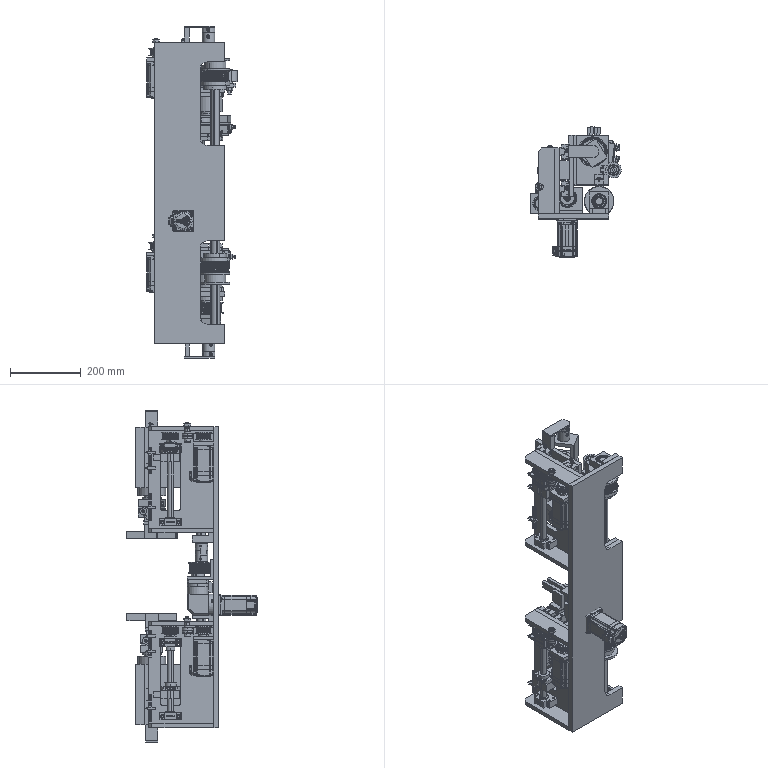Part | SolidWorks | features CompositeCurve 3, InContextFeatHolder 2 | 278 solids | 22008 faces | volume 10593540 mm3 | cylinder 9335 | plane 8631 | spline 2093 | cone 1921 | torus 28 | commonest cylinder face diameters 1.1 x904 0.5 x863 6.55 x798 3 x570 1 x406 2 x343